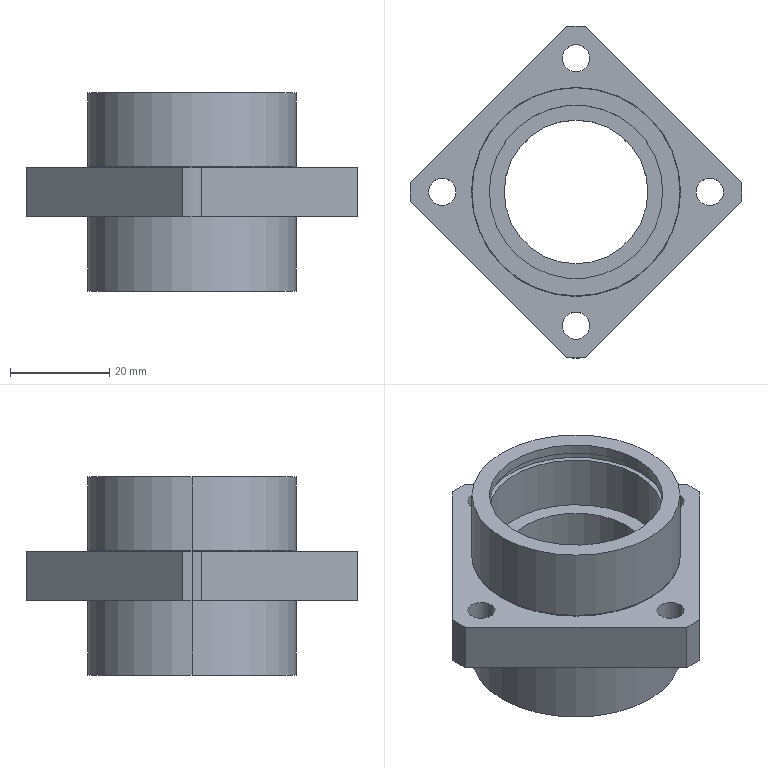Part | STEP file | HI_BFU71-6202ZZ-L40-S15S1^BFU71-6202ZZ-L40-S15_Idler roller assembly (direct encoder) | 1 solid | 59 faces | box 67 x 67 x 40 mm | volume 28798 mm3 | cylinder 39 | plane 18 | torus 2 | commonest cylinder face diameters 5.5 x8 9.5 x8 35 x8 67 x5 37 x4 42 x4